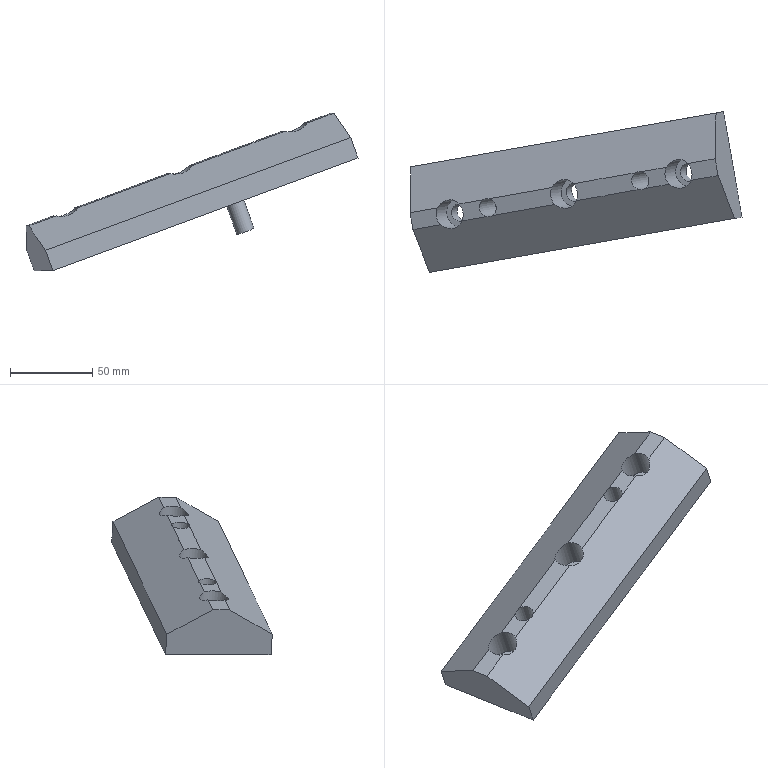Part | NX | features solid 2 | 1 solid | 28 faces | box 201.397 x 97.434 x 95.655 mm | volume 270921 mm3 | plane 17 | cylinder 11 | commonest cylinder face diameters 11 x8 17.5 x3
STEP:
#1=CARTESIAN_POINT('',(972.407,367.24,-198.041));
#2=VERTEX_POINT('',#1);
#3=CARTESIAN_POINT('',(987.359,369.877,-192.515));
#4=VERTEX_POINT('',#3);
#5=CARTESIAN_POINT('',(873.35,349.774,-234.651));
#6=DIRECTION('',(0.9254,0.1632,0.342));
#7=VECTOR('',#6,1000.);
#8=LINE('',#5,#7);
#9=EDGE_CURVE('',#2,#4,#8,.T.);
#10=ORIENTED_EDGE('',*,*,#9,.F.);
#11=CARTESIAN_POINT('',(974.212,357.006,-198.041));
#12=VERTEX_POINT('',#11);
#13=CARTESIAN_POINT('',(966.794,360.974,-200.449));
#14=DIRECTION('',(0.3368,0.05939,-0.9397));
#15=DIRECTION('',(-0.9254,-0.1632,-0.342));
#16=AXIS2_PLACEMENT_3D('',#13,#14,#15);
#17=CIRCLE('',#16,8.75);
#18=EDGE_CURVE('',#2,#12,#17,.T.);
#19=ORIENTED_EDGE('',*,*,#18,.T.);
#20=CARTESIAN_POINT('',(989.164,359.642,-192.515));
#21=VERTEX_POINT('',#20);
#22=CARTESIAN_POINT('',(875.155,339.54,-234.651));
#23=DIRECTION('',(0.9254,0.1632,0.342));
#24=VECTOR('',#23,1000.);
#25=LINE('',#22,#24);
#26=EDGE_CURVE('',#12,#21,#25,.T.);
#27=ORIENTED_EDGE('',*,*,#26,.T.);
#28=CARTESIAN_POINT('',(992.5,360.231,-191.282));
#29=VERTEX_POINT('',#28);
#30=CARTESIAN_POINT('',(989.93,365.054,-191.898));
#31=DIRECTION('',(-0.3368,-0.05939,0.9397));
#32=DIRECTION('',(0.9414,0.,0.3374));
#33=AXIS2_PLACEMENT_3D('',#30,#31,#32);
#34=CIRCLE('',#33,5.5);
#35=EDGE_CURVE('',#21,#29,#34,.T.);
#36=ORIENTED_EDGE('',*,*,#35,.T.);
#37=CARTESIAN_POINT('',(1012.299,363.722,-183.964));
#38=VERTEX_POINT('',#37);
#39=CARTESIAN_POINT('',(875.155,339.54,-234.651));
#40=DIRECTION('',(0.9254,0.1632,0.342));
#41=VECTOR('',#40,1000.);
#42=LINE('',#39,#41);
#43=EDGE_CURVE('',#29,#38,#42,.T.);
#44=ORIENTED_EDGE('',*,*,#43,.T.);
#45=CARTESIAN_POINT('',(1010.495,373.956,-183.964));
#46=VERTEX_POINT('',#45);
#47=CARTESIAN_POINT('',(1013.065,369.133,-183.348));
#48=DIRECTION('',(-0.3368,-0.05939,0.9397));
#49=DIRECTION('',(0.9254,0.1632,0.342));
#50=AXIS2_PLACEMENT_3D('',#47,#48,#49);
#51=CIRCLE('',#50,5.5);
#52=EDGE_CURVE('',#46,#38,#51,.T.);
#53=ORIENTED_EDGE('',*,*,#52,.F.);
#54=CARTESIAN_POINT('',(990.696,370.465,-191.282));
#55=VERTEX_POINT('',#54);
#56=CARTESIAN_POINT('',(873.35,349.774,-234.651));
#57=DIRECTION('',(0.9254,0.1632,0.342));
#58=VECTOR('',#57,1000.);
#59=LINE('',#56,#58);
#60=EDGE_CURVE('',#55,#46,#59,.T.);
#61=ORIENTED_EDGE('',*,*,#60,.F.);
#62=CARTESIAN_POINT('',(989.93,365.054,-191.898));
#63=DIRECTION('',(-0.3368,-0.05939,0.9397));
#64=DIRECTION('',(0.9414,0.,0.3374));
#65=AXIS2_PLACEMENT_3D('',#62,#63,#64);
#66=CIRCLE('',#65,5.5);
#67=EDGE_CURVE('',#55,#4,#66,.T.);
#68=ORIENTED_EDGE('',*,*,#67,.T.);
#69=EDGE_LOOP('',(#10,#19,#27,#36,#44,#53,#61,#68));
#70=FACE_BOUND('',#69,.T.);
#71=CARTESIAN_POINT('',(875.155,339.54,-234.651));
#72=DIRECTION('',(-0.3368,-0.05939,0.9397));
#73=DIRECTION('',(-0.9254,-0.1632,-0.342));
#74=AXIS2_PLACEMENT_3D('',#71,#72,#73);
#75=PLANE('',#74);
#76=ADVANCED_FACE('',(#70),#75,.T.);
#77=CARTESIAN_POINT('',(1051.058,375.832,-200.167));
#78=VERTEX_POINT('',#77);
#79=CARTESIAN_POINT('',(1045.969,374.935,-202.048));
#80=DIRECTION('',(0.3368,0.05939,-0.9397));
#81=DIRECTION('',(0.9254,0.1632,0.342));
#82=AXIS2_PLACEMENT_3D('',#79,#80,#81);
#83=CIRCLE('',#82,5.5);
#84=EDGE_CURVE('',#78,#78,#83,.T.);
#85=ORIENTED_EDGE('',*,*,#84,.F.);
#86=EDGE_LOOP('',(#85));
#87=FACE_BOUND('',#86,.T.);
#88=CARTESIAN_POINT('',(1027.923,371.753,-208.718));
#89=VERTEX_POINT('',#88);
#90=CARTESIAN_POINT('',(1022.833,370.855,-210.599));
#91=DIRECTION('',(-0.3368,-0.05939,0.9397));
#92=DIRECTION('',(0.9254,0.1632,0.342));
#93=AXIS2_PLACEMENT_3D('',#90,#91,#92);
#94=CIRCLE('',#93,5.5);
#95=EDGE_CURVE('',#89,#89,#94,.T.);
#96=ORIENTED_EDGE('',*,*,#95,.T.);
#97=EDGE_LOOP('',(#96));
#98=FACE_BOUND('',#97,.T.);
#99=CARTESIAN_POINT('',(981.652,363.594,-225.819));
#100=VERTEX_POINT('',#99);
#101=CARTESIAN_POINT('',(976.562,362.697,-227.7));
#102=DIRECTION('',(0.3368,0.05939,-0.9397));
#103=DIRECTION('',(0.9254,0.1632,0.342));
#104=AXIS2_PLACEMENT_3D('',#101,#102,#103);
#105=CIRCLE('',#104,5.5);
#106=EDGE_CURVE('',#100,#100,#105,.T.);
#107=ORIENTED_EDGE('',*,*,#106,.F.);
#108=EDGE_LOOP('',(#107));
#109=FACE_BOUND('',#108,.T.);
#110=CARTESIAN_POINT('',(889.664,314.373,-261.902));
#111=VERTEX_POINT('',#110);
#112=CARTESIAN_POINT('',(1074.747,347.008,-193.498));
#113=VERTEX_POINT('',#112);
#114=CARTESIAN_POINT('',(889.664,314.373,-261.902));
#115=DIRECTION('',(0.9254,0.1632,0.342));
#116=VECTOR('',#115,1000.);
#117=LINE('',#114,#116);
#118=EDGE_CURVE('',#111,#113,#117,.T.);
#119=ORIENTED_EDGE('',*,*,#118,.F.);
#120=CARTESIAN_POINT('',(878.377,378.385,-261.902));
#121=VERTEX_POINT('',#120);
#122=CARTESIAN_POINT('',(889.664,314.373,-261.902));
#123=DIRECTION('',(-0.1736,0.9848,0.));
#124=VECTOR('',#123,1000.);
#125=LINE('',#122,#124);
#126=EDGE_CURVE('',#111,#121,#125,.T.);
#127=ORIENTED_EDGE('',*,*,#126,.T.);
#128=CARTESIAN_POINT('',(1063.46,411.021,-193.498));
#129=VERTEX_POINT('',#128);
#130=CARTESIAN_POINT('',(878.377,378.385,-261.902));
#131=DIRECTION('',(0.9254,0.1632,0.342));
#132=VECTOR('',#131,1000.);
#133=LINE('',#130,#132);
#134=EDGE_CURVE('',#121,#129,#133,.T.);
#135=ORIENTED_EDGE('',*,*,#134,.T.);
#136=CARTESIAN_POINT('',(1074.747,347.008,-193.498));
#137=DIRECTION('',(-0.1736,0.9848,0.));
#138=VECTOR('',#137,1000.);
#139=LINE('',#136,#138);
#140=EDGE_CURVE('',#113,#129,#139,.T.);
#141=ORIENTED_EDGE('',*,*,#140,.F.);
#142=EDGE_LOOP('',(#119,#127,#135,#141));
#143=FACE_BOUND('',#142,.T.);
#144=CARTESIAN_POINT('',(935.381,355.435,-242.92));
#145=VERTEX_POINT('',#144);
#146=CARTESIAN_POINT('',(930.291,354.538,-244.801));
#147=DIRECTION('',(-0.3368,-0.05939,0.9397));
#148=DIRECTION('',(0.9254,0.1632,0.342));
#149=AXIS2_PLACEMENT_3D('',#146,#147,#148);
#150=CIRCLE('',#149,5.5);
#151=EDGE_CURVE('',#145,#145,#150,.T.);
#152=ORIENTED_EDGE('',*,*,#151,.T.);
#153=EDGE_LOOP('',(#152));
#154=FACE_BOUND('',#153,.T.);
#155=CARTESIAN_POINT('',(912.246,351.356,-251.47));
#156=VERTEX_POINT('',#155);
#157=CARTESIAN_POINT('',(907.156,350.459,-253.351));
#158=DIRECTION('',(0.3368,0.05939,-0.9397));
#159=DIRECTION('',(0.9254,0.1632,0.342));
#160=AXIS2_PLACEMENT_3D('',#157,#158,#159);
#161=CIRCLE('',#160,5.5);
#162=EDGE_CURVE('',#156,#156,#161,.T.);
#163=ORIENTED_EDGE('',*,*,#162,.F.);
#164=EDGE_LOOP('',(#163));
#165=FACE_BOUND('',#164,.T.);
#166=CARTESIAN_POINT('',(1004.875,366.776,-217.294));
#167=VERTEX_POINT('',#166);
#168=CARTESIAN_POINT('',(999.698,366.776,-219.149));
#169=DIRECTION('',(-0.3368,-0.05939,0.9397));
#170=DIRECTION('',(0.9414,0.,0.3374));
#171=AXIS2_PLACEMENT_3D('',#168,#169,#170);
#172=CIRCLE('',#171,5.5);
#173=EDGE_CURVE('',#167,#167,#172,.T.);
#174=ORIENTED_EDGE('',*,*,#173,.T.);
#175=EDGE_LOOP('',(#174));
#176=FACE_BOUND('',#175,.T.);
#177=CARTESIAN_POINT('',(889.664,314.373,-261.902));
#178=DIRECTION('',(-0.3368,-0.05939,0.9397));
#179=DIRECTION('',(0.1736,-0.9848,0.));
#180=AXIS2_PLACEMENT_3D('',#177,#178,#179);
#181=PLANE('',#180);
#182=ADVANCED_FACE('',(#87,#98,#109,#143,#154,#165,#176),#181,.F.);
#183=ORIENTED_EDGE('',*,*,#60,.T.);
#184=CARTESIAN_POINT('',(1013.831,374.545,-182.731));
#185=VERTEX_POINT('',#184);
#186=CARTESIAN_POINT('',(1012.055,368.955,-180.529));
#187=DIRECTION('',(0.3785,-0.441,-0.8138));
#188=DIRECTION('',(0.01803,0.8826,-0.4698));
#189=AXIS2_PLACEMENT_3D('',#186,#187,#188);
#190=ELLIPSE('',#189,6.351,5.5);
#191=EDGE_CURVE('',#46,#185,#190,.T.);
#192=ORIENTED_EDGE('',*,*,#191,.T.);
#193=CARTESIAN_POINT('',(1028.783,377.181,-177.205));
#194=VERTEX_POINT('',#193);
#195=CARTESIAN_POINT('',(873.35,349.774,-234.651));
#196=DIRECTION('',(0.9254,0.1632,0.342));
#197=VECTOR('',#196,1000.);
#198=LINE('',#195,#197);
#199=EDGE_CURVE('',#185,#194,#198,.T.);
#200=ORIENTED_EDGE('',*,*,#199,.T.);
#201=CARTESIAN_POINT('',(1041.813,379.479,-172.389));
#202=VERTEX_POINT('',#201);
#203=CARTESIAN_POINT('',(1035.19,373.034,-171.978));
#204=DIRECTION('',(0.3785,-0.441,-0.8138));
#205=DIRECTION('',(0.01803,0.8826,-0.4698));
#206=AXIS2_PLACEMENT_3D('',#203,#204,#205);
#207=ELLIPSE('',#206,10.104,8.75);
#208=EDGE_CURVE('',#194,#202,#207,.T.);
#209=ORIENTED_EDGE('',*,*,#208,.T.);
#210=CARTESIAN_POINT('',(1058.434,382.409,-166.247));
#211=VERTEX_POINT('',#210);
#212=CARTESIAN_POINT('',(873.35,349.774,-234.651));
#213=DIRECTION('',(0.9254,0.1632,0.342));
#214=VECTOR('',#213,1000.);
#215=LINE('',#212,#214);
#216=EDGE_CURVE('',#202,#211,#215,.T.);
#217=ORIENTED_EDGE('',*,*,#216,.T.);
#218=CARTESIAN_POINT('',(1059.002,410.234,-181.06));
#219=VERTEX_POINT('',#218);
#220=CARTESIAN_POINT('',(1058.434,382.409,-166.247));
#221=DIRECTION('',(0.01803,0.8826,-0.4698));
#222=VECTOR('',#221,1000.);
#223=LINE('',#220,#222);
#224=EDGE_CURVE('',#211,#219,#223,.T.);
#225=ORIENTED_EDGE('',*,*,#224,.T.);
#226=CARTESIAN_POINT('',(873.919,377.599,-249.464));
#227=VERTEX_POINT('',#226);
#228=CARTESIAN_POINT('',(873.919,377.599,-249.464));
#229=DIRECTION('',(0.9254,0.1632,0.342));
#230=VECTOR('',#229,1000.);
#231=LINE('',#228,#230);
#232=EDGE_CURVE('',#227,#219,#231,.T.);
#233=ORIENTED_EDGE('',*,*,#232,.F.);
#234=CARTESIAN_POINT('',(873.35,349.774,-234.651));
#235=VERTEX_POINT('',#234);
#236=CARTESIAN_POINT('',(873.35,349.774,-234.651));
#237=DIRECTION('',(0.01803,0.8826,-0.4698));
#238=VECTOR('',#237,1000.);
#239=LINE('',#236,#238);
#240=EDGE_CURVE('',#235,#227,#239,.T.);
#241=ORIENTED_EDGE('',*,*,#240,.F.);
#242=CARTESIAN_POINT('',(889.971,352.705,-228.508));
#243=VERTEX_POINT('',#242);
#244=CARTESIAN_POINT('',(873.35,349.774,-234.651));
#245=DIRECTION('',(0.9254,0.1632,0.342));
#246=VECTOR('',#245,1000.);
#247=LINE('',#244,#246);
#248=EDGE_CURVE('',#235,#243,#247,.T.);
#249=ORIENTED_EDGE('',*,*,#248,.T.);
#250=CARTESIAN_POINT('',(903.001,355.002,-223.692));
#251=VERTEX_POINT('',#250);
#252=CARTESIAN_POINT('',(896.378,348.558,-223.281));
#253=DIRECTION('',(0.3785,-0.441,-0.8138));
#254=DIRECTION('',(0.01803,0.8826,-0.4698));
#255=AXIS2_PLACEMENT_3D('',#252,#253,#254);
#256=ELLIPSE('',#255,10.104,8.75);
#257=EDGE_CURVE('',#243,#251,#256,.T.);
#258=ORIENTED_EDGE('',*,*,#257,.T.);
#259=CARTESIAN_POINT('',(917.953,357.639,-218.166));
#260=VERTEX_POINT('',#259);
#261=CARTESIAN_POINT('',(873.35,349.774,-234.651));
#262=DIRECTION('',(0.9254,0.1632,0.342));
#263=VECTOR('',#262,1000.);
#264=LINE('',#261,#263);
#265=EDGE_CURVE('',#251,#260,#264,.T.);
#266=ORIENTED_EDGE('',*,*,#265,.T.);
#267=CARTESIAN_POINT('',(921.29,358.227,-216.933));
#268=VERTEX_POINT('',#267);
#269=CARTESIAN_POINT('',(919.513,352.637,-214.731));
#270=DIRECTION('',(0.3785,-0.441,-0.8138));
#271=DIRECTION('',(0.01803,0.8826,-0.4698));
#272=AXIS2_PLACEMENT_3D('',#269,#270,#271);
#273=ELLIPSE('',#272,6.351,5.5);
#274=EDGE_CURVE('',#260,#268,#273,.T.);
#275=ORIENTED_EDGE('',*,*,#274,.T.);
#276=CARTESIAN_POINT('',(959.377,364.943,-202.857));
#277=VERTEX_POINT('',#276);
#278=CARTESIAN_POINT('',(873.35,349.774,-234.651));
#279=DIRECTION('',(0.9254,0.1632,0.342));
#280=VECTOR('',#279,1000.);
#281=LINE('',#278,#280);
#282=EDGE_CURVE('',#268,#277,#281,.T.);
#283=ORIENTED_EDGE('',*,*,#282,.T.);
#284=CARTESIAN_POINT('',(965.784,360.796,-197.63));
#285=DIRECTION('',(0.3785,-0.441,-0.8138));
#286=DIRECTION('',(0.01803,0.8826,-0.4698));
#287=AXIS2_PLACEMENT_3D('',#284,#285,#286);
#288=ELLIPSE('',#287,10.104,8.75);
#289=EDGE_CURVE('',#277,#2,#288,.T.);
#290=ORIENTED_EDGE('',*,*,#289,.T.);
#291=ORIENTED_EDGE('',*,*,#9,.T.);
#292=CARTESIAN_POINT('',(988.919,364.876,-189.079));
#293=DIRECTION('',(-0.3785,0.441,0.8138));
#294=DIRECTION('',(0.01803,0.8826,-0.4698));
#295=AXIS2_PLACEMENT_3D('',#292,#293,#294);
#296=ELLIPSE('',#295,6.351,5.5);
#297=EDGE_CURVE('',#4,#55,#296,.F.);
#298=ORIENTED_EDGE('',*,*,#297,.T.);
#299=EDGE_LOOP('',(#183,#192,#200,#209,#217,#225,#233,#241,#249,#258,#266,#275,#283,#290,#291,#298));
#300=FACE_BOUND('',#299,.T.);
#301=CARTESIAN_POINT('',(873.35,349.774,-234.651));
#302=DIRECTION('',(-0.3785,0.441,0.8138));
#303=DIRECTION('',(-0.01803,-0.8826,0.4698));
#304=AXIS2_PLACEMENT_3D('',#301,#302,#303);
#305=PLANE('',#304);
#306=ADVANCED_FACE('',(#300),#305,.T.);
#307=ORIENTED_EDGE('',*,*,#26,.F.);
#308=CARTESIAN_POINT('',(961.182,354.708,-202.857));
#309=VERTEX_POINT('',#308);
#310=CARTESIAN_POINT('',(965.784,360.796,-197.63));
#311=DIRECTION('',(-0.2049,-0.5438,0.8138));
#312=DIRECTION('',(0.3188,-0.8232,-0.4698));
#313=AXIS2_PLACEMENT_3D('',#310,#311,#312);
#314=ELLIPSE('',#313,10.104,8.75);
#315=EDGE_CURVE('',#309,#12,#314,.T.);
#316=ORIENTED_EDGE('',*,*,#315,.F.);
#317=CARTESIAN_POINT('',(923.094,347.993,-216.933));
#318=VERTEX_POINT('',#317);
#319=CARTESIAN_POINT('',(875.155,339.54,-234.651));
#320=DIRECTION('',(0.9254,0.1632,0.342));
#321=VECTOR('',#320,1000.);
#322=LINE('',#319,#321);
#323=EDGE_CURVE('',#318,#309,#322,.T.);
#324=ORIENTED_EDGE('',*,*,#323,.F.);
#325=CARTESIAN_POINT('',(919.758,347.404,-218.166));
#326=VERTEX_POINT('',#325);
#327=CARTESIAN_POINT('',(919.513,352.637,-214.731));
#328=DIRECTION('',(-0.2049,-0.5438,0.8138));
#329=DIRECTION('',(0.3188,-0.8232,-0.4698));
#330=AXIS2_PLACEMENT_3D('',#327,#328,#329);
#331=ELLIPSE('',#330,6.351,5.5);
#332=EDGE_CURVE('',#326,#318,#331,.T.);
#333=ORIENTED_EDGE('',*,*,#332,.F.);
#334=CARTESIAN_POINT('',(904.805,344.768,-223.692));
#335=VERTEX_POINT('',#334);
#336=CARTESIAN_POINT('',(875.155,339.54,-234.651));
#337=DIRECTION('',(0.9254,0.1632,0.342));
#338=VECTOR('',#337,1000.);
#339=LINE('',#336,#338);
#340=EDGE_CURVE('',#335,#326,#339,.T.);
#341=ORIENTED_EDGE('',*,*,#340,.F.);
#342=CARTESIAN_POINT('',(891.775,342.47,-228.508));
#343=VERTEX_POINT('',#342);
#344=CARTESIAN_POINT('',(896.378,348.558,-223.281));
#345=DIRECTION('',(-0.2049,-0.5438,0.8138));
#346=DIRECTION('',(0.3188,-0.8232,-0.4698));
#347=AXIS2_PLACEMENT_3D('',#344,#345,#346);
#348=ELLIPSE('',#347,10.104,8.75);
#349=EDGE_CURVE('',#343,#335,#348,.T.);
#350=ORIENTED_EDGE('',*,*,#349,.F.);
#351=CARTESIAN_POINT('',(875.155,339.54,-234.651));
#352=VERTEX_POINT('',#351);
#353=CARTESIAN_POINT('',(875.155,339.54,-234.651));
#354=DIRECTION('',(0.9254,0.1632,0.342));
#355=VECTOR('',#354,1000.);
#356=LINE('',#353,#355);
#357=EDGE_CURVE('',#352,#343,#356,.T.);
#358=ORIENTED_EDGE('',*,*,#357,.F.);
#359=CARTESIAN_POINT('',(885.206,313.587,-249.464));
#360=VERTEX_POINT('',#359);
#361=CARTESIAN_POINT('',(875.155,339.54,-234.651));
#362=DIRECTION('',(0.3188,-0.8232,-0.4698));
#363=VECTOR('',#362,1000.);
#364=LINE('',#361,#363);
#365=EDGE_CURVE('',#352,#360,#364,.T.);
#366=ORIENTED_EDGE('',*,*,#365,.T.);
#367=CARTESIAN_POINT('',(1070.289,346.222,-181.06));
#368=VERTEX_POINT('',#367);
#369=CARTESIAN_POINT('',(885.206,313.587,-249.464));
#370=DIRECTION('',(0.9254,0.1632,0.342));
#371=VECTOR('',#370,1000.);
#372=LINE('',#369,#371);
#373=EDGE_CURVE('',#360,#368,#372,.T.);
#374=ORIENTED_EDGE('',*,*,#373,.T.);
#375=CARTESIAN_POINT('',(1060.238,372.175,-166.247));
#376=VERTEX_POINT('',#375);
#377=CARTESIAN_POINT('',(1060.238,372.175,-166.247));
#378=DIRECTION('',(0.3188,-0.8232,-0.4698));
#379=VECTOR('',#378,1000.);
#380=LINE('',#377,#379);
#381=EDGE_CURVE('',#376,#368,#380,.T.);
#382=ORIENTED_EDGE('',*,*,#381,.F.);
#383=CARTESIAN_POINT('',(1043.618,369.244,-172.389));
#384=VERTEX_POINT('',#383);
#385=CARTESIAN_POINT('',(875.155,339.54,-234.651));
#386=DIRECTION('',(0.9254,0.1632,0.342));
#387=VECTOR('',#386,1000.);
#388=LINE('',#385,#387);
#389=EDGE_CURVE('',#384,#376,#388,.T.);
#390=ORIENTED_EDGE('',*,*,#389,.F.);
#391=CARTESIAN_POINT('',(1030.588,366.947,-177.205));
#392=VERTEX_POINT('',#391);
#393=CARTESIAN_POINT('',(1035.19,373.034,-171.978));
#394=DIRECTION('',(-0.2049,-0.5438,0.8138));
#395=DIRECTION('',(0.3188,-0.8232,-0.4698));
#396=AXIS2_PLACEMENT_3D('',#393,#394,#395);
#397=ELLIPSE('',#396,10.104,8.75);
#398=EDGE_CURVE('',#392,#384,#397,.T.);
#399=ORIENTED_EDGE('',*,*,#398,.F.);
#400=CARTESIAN_POINT('',(1015.636,364.31,-182.731));
#401=VERTEX_POINT('',#400);
#402=CARTESIAN_POINT('',(875.155,339.54,-234.651));
#403=DIRECTION('',(0.9254,0.1632,0.342));
#404=VECTOR('',#403,1000.);
#405=LINE('',#402,#404);
#406=EDGE_CURVE('',#401,#392,#405,.T.);
#407=ORIENTED_EDGE('',*,*,#406,.F.);
#408=CARTESIAN_POINT('',(1012.055,368.955,-180.529));
#409=DIRECTION('',(-0.2049,-0.5438,0.8138));
#410=DIRECTION('',(0.3188,-0.8232,-0.4698));
#411=AXIS2_PLACEMENT_3D('',#408,#409,#410);
#412=ELLIPSE('',#411,6.351,5.5);
#413=EDGE_CURVE('',#38,#401,#412,.T.);
#414=ORIENTED_EDGE('',*,*,#413,.F.);
#415=ORIENTED_EDGE('',*,*,#43,.F.);
#416=CARTESIAN_POINT('',(988.919,364.876,-189.079));
#417=DIRECTION('',(-0.2049,-0.5438,0.8138));
#418=DIRECTION('',(0.3188,-0.8232,-0.4698));
#419=AXIS2_PLACEMENT_3D('',#416,#417,#418);
#420=ELLIPSE('',#419,6.351,5.5);
#421=EDGE_CURVE('',#29,#21,#420,.F.);
#422=ORIENTED_EDGE('',*,*,#421,.T.);
#423=EDGE_LOOP('',(#307,#316,#324,#333,#341,#350,#358,#366,#374,#382,#390,#399,#407,#414,#415,#422));
#424=FACE_BOUND('',#423,.T.);
#425=CARTESIAN_POINT('',(875.155,339.54,-234.651));
#426=DIRECTION('',(-0.2049,-0.5438,0.8138));
#427=DIRECTION('',(-0.3188,0.8232,0.4698));
#428=AXIS2_PLACEMENT_3D('',#425,#426,#427);
#429=PLANE('',#428);
#430=ADVANCED_FACE('',(#424),#429,.T.);
#431=CARTESIAN_POINT('',(966.794,360.974,-200.449));
#432=DIRECTION('',(-0.3368,-0.05939,0.9397));
#433=DIRECTION('',(0.9254,0.1632,0.342));
#434=AXIS2_PLACEMENT_3D('',#431,#432,#433);
#435=CIRCLE('',#434,8.75);
#436=EDGE_CURVE('',#277,#309,#435,.T.);
#437=ORIENTED_EDGE('',*,*,#436,.F.);
#438=ORIENTED_EDGE('',*,*,#282,.F.);
#439=CARTESIAN_POINT('',(920.524,352.816,-217.55));
#440=DIRECTION('',(-0.3368,-0.05939,0.9397));
#441=DIRECTION('',(0.9254,0.1632,0.342));
#442=AXIS2_PLACEMENT_3D('',#439,#440,#441);
#443=CIRCLE('',#442,5.5);
#444=EDGE_CURVE('',#318,#268,#443,.T.);
#445=ORIENTED_EDGE('',*,*,#444,.F.);
#446=ORIENTED_EDGE('',*,*,#323,.T.);
#447=EDGE_LOOP('',(#437,#438,#445,#446));
#448=FACE_BOUND('',#447,.T.);
#449=CARTESIAN_POINT('',(875.155,339.54,-234.651));
#450=DIRECTION('',(-0.3368,-0.05939,0.9397));
#451=DIRECTION('',(-0.9254,-0.1632,-0.342));
#452=AXIS2_PLACEMENT_3D('',#449,#450,#451);
#453=PLANE('',#452);
#454=ADVANCED_FACE('',(#448),#453,.T.);
#455=CARTESIAN_POINT('',(920.524,352.816,-217.55));
#456=DIRECTION('',(-0.3368,-0.05939,0.9397));
#457=DIRECTION('',(0.9254,0.1632,0.342));
#458=AXIS2_PLACEMENT_3D('',#455,#456,#457);
#459=CIRCLE('',#458,5.5);
#460=EDGE_CURVE('',#260,#326,#459,.T.);
#461=ORIENTED_EDGE('',*,*,#460,.F.);
#462=ORIENTED_EDGE('',*,*,#265,.F.);
#463=CARTESIAN_POINT('',(897.388,348.736,-226.1));
#464=DIRECTION('',(0.3368,0.05939,-0.9397));
#465=DIRECTION('',(-0.9254,-0.1632,-0.342));
#466=AXIS2_PLACEMENT_3D('',#463,#464,#465);
#467=CIRCLE('',#466,8.75);
#468=EDGE_CURVE('',#251,#335,#467,.T.);
#469=ORIENTED_EDGE('',*,*,#468,.T.);
#470=ORIENTED_EDGE('',*,*,#340,.T.);
#471=EDGE_LOOP('',(#461,#462,#469,#470));
#472=FACE_BOUND('',#471,.T.);
#473=CARTESIAN_POINT('',(875.155,339.54,-234.651));
#474=DIRECTION('',(-0.3368,-0.05939,0.9397));
#475=DIRECTION('',(-0.9254,-0.1632,-0.342));
#476=AXIS2_PLACEMENT_3D('',#473,#474,#475);
#477=PLANE('',#476);
#478=ADVANCED_FACE('',(#472),#477,.T.);
#479=CARTESIAN_POINT('',(1036.201,373.213,-174.797));
#480=DIRECTION('',(-0.3368,-0.05939,0.9397));
#481=DIRECTION('',(0.9254,0.1632,0.342));
#482=AXIS2_PLACEMENT_3D('',#479,#480,#481);
#483=CIRCLE('',#482,8.75);
#484=EDGE_CURVE('',#194,#392,#483,.T.);
#485=ORIENTED_EDGE('',*,*,#484,.F.);
#486=ORIENTED_EDGE('',*,*,#199,.F.);
#487=CARTESIAN_POINT('',(1013.065,369.133,-183.348));
#488=DIRECTION('',(0.3368,0.05939,-0.9397));
#489=DIRECTION('',(-0.9254,-0.1632,-0.342));
#490=AXIS2_PLACEMENT_3D('',#487,#488,#489);
#491=CIRCLE('',#490,5.5);
#492=EDGE_CURVE('',#185,#401,#491,.T.);
#493=ORIENTED_EDGE('',*,*,#492,.T.);
#494=ORIENTED_EDGE('',*,*,#406,.T.);
#495=EDGE_LOOP('',(#485,#486,#493,#494));
#496=FACE_BOUND('',#495,.T.);
#497=CARTESIAN_POINT('',(875.155,339.54,-234.651));
#498=DIRECTION('',(-0.3368,-0.05939,0.9397));
#499=DIRECTION('',(-0.9254,-0.1632,-0.342));
#500=AXIS2_PLACEMENT_3D('',#497,#498,#499);
#501=PLANE('',#500);
#502=ADVANCED_FACE('',(#496),#501,.T.);
#503=CARTESIAN_POINT('',(1060.238,372.175,-166.247));
#504=DIRECTION('',(-0.1736,0.9848,0.));
#505=VECTOR('',#504,1000.);
#506=LINE('',#503,#505);
#507=EDGE_CURVE('',#376,#211,#506,.T.);
#508=ORIENTED_EDGE('',*,*,#507,.T.);
#509=ORIENTED_EDGE('',*,*,#216,.F.);
#510=CARTESIAN_POINT('',(1036.201,373.213,-174.797));
#511=DIRECTION('',(0.3368,0.05939,-0.9397));
#512=DIRECTION('',(-0.9254,-0.1632,-0.342));
#513=AXIS2_PLACEMENT_3D('',#510,#511,#512);
#514=CIRCLE('',#513,8.75);
#515=EDGE_CURVE('',#202,#384,#514,.T.);
#516=ORIENTED_EDGE('',*,*,#515,.T.);
#517=ORIENTED_EDGE('',*,*,#389,.T.);
#518=EDGE_LOOP('',(#508,#509,#516,#517));
#519=FACE_BOUND('',#518,.T.);
#520=CARTESIAN_POINT('',(875.155,339.54,-234.651));
#521=DIRECTION('',(-0.3368,-0.05939,0.9397));
#522=DIRECTION('',(-0.9254,-0.1632,-0.342));
#523=AXIS2_PLACEMENT_3D('',#520,#521,#522);
#524=PLANE('',#523);
#525=ADVANCED_FACE('',(#519),#524,.T.);
#526=CARTESIAN_POINT('',(897.388,348.736,-226.1));
#527=DIRECTION('',(-0.3368,-0.05939,0.9397));
#528=DIRECTION('',(0.9254,0.1632,0.342));
#529=AXIS2_PLACEMENT_3D('',#526,#527,#528);
#530=CIRCLE('',#529,8.75);
#531=EDGE_CURVE('',#243,#343,#530,.T.);
#532=ORIENTED_EDGE('',*,*,#531,.F.);
#533=ORIENTED_EDGE('',*,*,#248,.F.);
#534=CARTESIAN_POINT('',(875.155,339.54,-234.651));
#535=DIRECTION('',(-0.1736,0.9848,0.));
#536=VECTOR('',#535,1000.);
#537=LINE('',#534,#536);
#538=EDGE_CURVE('',#352,#235,#537,.T.);
#539=ORIENTED_EDGE('',*,*,#538,.F.);
#540=ORIENTED_EDGE('',*,*,#357,.T.);
#541=EDGE_LOOP('',(#532,#533,#539,#540));
#542=FACE_BOUND('',#541,.T.);
#543=CARTESIAN_POINT('',(875.155,339.54,-234.651));
#544=DIRECTION('',(-0.3368,-0.05939,0.9397));
#545=DIRECTION('',(-0.9254,-0.1632,-0.342));
#546=AXIS2_PLACEMENT_3D('',#543,#544,#545);
#547=PLANE('',#546);
#548=ADVANCED_FACE('',(#542),#547,.T.);
#549=ORIENTED_EDGE('',*,*,#538,.T.);
#550=ORIENTED_EDGE('',*,*,#240,.T.);
#551=CARTESIAN_POINT('',(883.429,379.276,-275.997));
#552=DIRECTION('',(-0.3368,-0.05939,0.9397));
#553=VECTOR('',#552,1000.);
#554=LINE('',#551,#553);
#555=EDGE_CURVE('',#121,#227,#554,.T.);
#556=ORIENTED_EDGE('',*,*,#555,.F.);
#557=ORIENTED_EDGE('',*,*,#126,.F.);
#558=CARTESIAN_POINT('',(894.717,315.264,-275.997));
#559=DIRECTION('',(-0.3368,-0.05939,0.9397));
#560=VECTOR('',#559,1000.);
#561=LINE('',#558,#560);
#562=EDGE_CURVE('',#111,#360,#561,.T.);
#563=ORIENTED_EDGE('',*,*,#562,.T.);
#564=ORIENTED_EDGE('',*,*,#365,.F.);
#565=EDGE_LOOP('',(#549,#550,#556,#557,#563,#564));
#566=FACE_BOUND('',#565,.T.);
#567=CARTESIAN_POINT('',(873.242,344.479,-231.832));
#568=DIRECTION('',(-0.9254,-0.1632,-0.342));
#569=DIRECTION('',(0.3368,0.05939,-0.9397));
#570=AXIS2_PLACEMENT_3D('',#567,#568,#569);
#571=PLANE('',#570);
#572=ADVANCED_FACE('',(#566),#571,.T.);
#573=ORIENTED_EDGE('',*,*,#507,.F.);
#574=ORIENTED_EDGE('',*,*,#381,.T.);
#575=CARTESIAN_POINT('',(1079.8,347.899,-207.593));
#576=DIRECTION('',(-0.3368,-0.05939,0.9397));
#577=VECTOR('',#576,1000.);
#578=LINE('',#575,#577);
#579=EDGE_CURVE('',#113,#368,#578,.T.);
#580=ORIENTED_EDGE('',*,*,#579,.F.);
#581=ORIENTED_EDGE('',*,*,#140,.T.);
#582=CARTESIAN_POINT('',(1068.513,411.911,-207.593));
#583=DIRECTION('',(-0.3368,-0.05939,0.9397));
#584=VECTOR('',#583,1000.);
#585=LINE('',#582,#584);
#586=EDGE_CURVE('',#129,#219,#585,.T.);
#587=ORIENTED_EDGE('',*,*,#586,.T.);
#588=ORIENTED_EDGE('',*,*,#224,.F.);
#589=EDGE_LOOP('',(#573,#574,#580,#581,#587,#588));
#590=FACE_BOUND('',#589,.T.);
#591=CARTESIAN_POINT('',(1058.326,377.114,-163.428));
#592=DIRECTION('',(-0.9254,-0.1632,-0.342));
#593=DIRECTION('',(0.3368,0.05939,-0.9397));
#594=AXIS2_PLACEMENT_3D('',#591,#592,#593);
#595=PLANE('',#594);
#596=ADVANCED_FACE('',(#590),#595,.F.);
#597=ORIENTED_EDGE('',*,*,#84,.T.);
#598=EDGE_LOOP('',(#597));
#599=FACE_BOUND('',#598,.T.);
#600=CARTESIAN_POINT('',(1037.423,374.341,-194.507));
#601=VERTEX_POINT('',#600);
#602=CARTESIAN_POINT('',(1042.6,374.341,-192.651));
#603=DIRECTION('',(0.3368,0.05939,-0.9397));
#604=DIRECTION('',(-0.9414,0.,-0.3374));
#605=AXIS2_PLACEMENT_3D('',#602,#603,#604);
#606=CIRCLE('',#605,5.5);
#607=EDGE_CURVE('',#601,#601,#606,.F.);
#608=ORIENTED_EDGE('',*,*,#607,.T.);
#609=EDGE_LOOP('',(#608));
#610=FACE_BOUND('',#609,.T.);
#611=CARTESIAN_POINT('',(1052.031,376.004,-218.963));
#612=DIRECTION('',(0.3368,0.05939,-0.9397));
#613=DIRECTION('',(0.9254,0.1632,0.342));
#614=AXIS2_PLACEMENT_3D('',#611,#612,#613);
#615=CYLINDRICAL_SURFACE('',#614,5.5);
#616=ADVANCED_FACE('',(#599,#610),#615,.F.);
#617=ORIENTED_EDGE('',*,*,#607,.F.);
#618=EDGE_LOOP('',(#617));
#619=FACE_BOUND('',#618,.T.);
#620=CARTESIAN_POINT('',(1034.363,374.341,-195.604));
#621=VERTEX_POINT('',#620);
#622=CARTESIAN_POINT('',(1042.6,374.341,-192.651));
#623=DIRECTION('',(0.3368,0.05939,-0.9397));
#624=DIRECTION('',(-0.9414,0.,-0.3374));
#625=AXIS2_PLACEMENT_3D('',#622,#623,#624);
#626=CIRCLE('',#625,8.75);
#627=EDGE_CURVE('',#621,#621,#626,.F.);
#628=ORIENTED_EDGE('',*,*,#627,.T.);
#629=EDGE_LOOP('',(#628));
#630=FACE_BOUND('',#629,.T.);
#631=CARTESIAN_POINT('',(996.329,366.182,-209.752));
#632=DIRECTION('',(0.3368,0.05939,-0.9397));
#633=DIRECTION('',(0.9254,0.1632,0.342));
#634=AXIS2_PLACEMENT_3D('',#631,#632,#633);
#635=PLANE('',#634);
#636=ADVANCED_FACE('',(#619,#630),#635,.F.);
#637=ORIENTED_EDGE('',*,*,#627,.F.);
#638=EDGE_LOOP('',(#637));
#639=FACE_BOUND('',#638,.T.);
#640=ORIENTED_EDGE('',*,*,#484,.T.);
#641=ORIENTED_EDGE('',*,*,#398,.T.);
#642=ORIENTED_EDGE('',*,*,#515,.F.);
#643=ORIENTED_EDGE('',*,*,#208,.F.);
#644=EDGE_LOOP('',(#640,#641,#642,#643));
#645=FACE_BOUND('',#644,.T.);
#646=CARTESIAN_POINT('',(1036.201,373.213,-174.797));
#647=DIRECTION('',(0.3368,0.05939,-0.9397));
#648=DIRECTION('',(0.9254,0.1632,0.342));
#649=AXIS2_PLACEMENT_3D('',#646,#647,#648);
#650=CYLINDRICAL_SURFACE('',#649,8.75);
#651=ADVANCED_FACE('',(#639,#645),#650,.F.);
#652=ORIENTED_EDGE('',*,*,#95,.F.);
#653=EDGE_LOOP('',(#652));
#654=FACE_BOUND('',#653,.T.);
#655=ORIENTED_EDGE('',*,*,#52,.T.);
#656=ORIENTED_EDGE('',*,*,#413,.T.);
#657=ORIENTED_EDGE('',*,*,#492,.F.);
#658=ORIENTED_EDGE('',*,*,#191,.F.);
#659=EDGE_LOOP('',(#655,#656,#657,#658));
#660=FACE_BOUND('',#659,.T.);
#661=CARTESIAN_POINT('',(1013.065,369.133,-183.348));
#662=DIRECTION('',(0.3368,0.05939,-0.9397));
#663=DIRECTION('',(0.9254,0.1632,0.342));
#664=AXIS2_PLACEMENT_3D('',#661,#662,#663);
#665=CYLINDRICAL_SURFACE('',#664,5.5);
#666=ADVANCED_FACE('',(#654,#660),#665,.F.);
#667=ORIENTED_EDGE('',*,*,#106,.T.);
#668=EDGE_LOOP('',(#667));
#669=FACE_BOUND('',#668,.T.);
#670=CARTESIAN_POINT('',(968.017,362.103,-220.159));
#671=VERTEX_POINT('',#670);
#672=CARTESIAN_POINT('',(973.194,362.103,-218.303));
#673=DIRECTION('',(0.3368,0.05939,-0.9397));
#674=DIRECTION('',(-0.9414,0.,-0.3374));
#675=AXIS2_PLACEMENT_3D('',#672,#673,#674);
#676=CIRCLE('',#675,5.5);
#677=EDGE_CURVE('',#671,#671,#676,.F.);
#678=ORIENTED_EDGE('',*,*,#677,.T.);
#679=EDGE_LOOP('',(#678));
#680=FACE_BOUND('',#679,.T.);
#681=CARTESIAN_POINT('',(982.625,363.766,-244.614));
#682=DIRECTION('',(0.3368,0.05939,-0.9397));
#683=DIRECTION('',(0.9254,0.1632,0.342));
#684=AXIS2_PLACEMENT_3D('',#681,#682,#683);
#685=CYLINDRICAL_SURFACE('',#684,5.5);
#686=ADVANCED_FACE('',(#669,#680),#685,.F.);
#687=ORIENTED_EDGE('',*,*,#677,.F.);
#688=EDGE_LOOP('',(#687));
#689=FACE_BOUND('',#688,.T.);
#690=CARTESIAN_POINT('',(964.957,362.103,-221.255));
#691=VERTEX_POINT('',#690);
#692=CARTESIAN_POINT('',(973.194,362.103,-218.303));
#693=DIRECTION('',(0.3368,0.05939,-0.9397));
#694=DIRECTION('',(-0.9414,0.,-0.3374));
#695=AXIS2_PLACEMENT_3D('',#692,#693,#694);
#696=CIRCLE('',#695,8.75);
#697=EDGE_CURVE('',#691,#691,#696,.F.);
#698=ORIENTED_EDGE('',*,*,#697,.T.);
#699=EDGE_LOOP('',(#698));
#700=FACE_BOUND('',#699,.T.);
#701=CARTESIAN_POINT('',(973.194,362.103,-218.303));
#702=DIRECTION('',(0.3368,0.05939,-0.9397));
#703=DIRECTION('',(0.9254,0.1632,0.342));
#704=AXIS2_PLACEMENT_3D('',#701,#702,#703);
#705=PLANE('',#704);
#706=ADVANCED_FACE('',(#689,#700),#705,.F.);
#707=ORIENTED_EDGE('',*,*,#697,.F.);
#708=EDGE_LOOP('',(#707));
#709=FACE_BOUND('',#708,.T.);
#710=ORIENTED_EDGE('',*,*,#436,.T.);
#711=ORIENTED_EDGE('',*,*,#315,.T.);
#712=ORIENTED_EDGE('',*,*,#18,.F.);
#713=ORIENTED_EDGE('',*,*,#289,.F.);
#714=EDGE_LOOP('',(#710,#711,#712,#713));
#715=FACE_BOUND('',#714,.T.);
#716=CARTESIAN_POINT('',(966.794,360.974,-200.449));
#717=DIRECTION('',(0.3368,0.05939,-0.9397));
#718=DIRECTION('',(0.9254,0.1632,0.342));
#719=AXIS2_PLACEMENT_3D('',#716,#717,#718);
#720=CYLINDRICAL_SURFACE('',#719,8.75);
#721=ADVANCED_FACE('',(#709,#715),#720,.F.);
#722=CARTESIAN_POINT('',(898.61,349.865,-245.81));
#723=VERTEX_POINT('',#722);
#724=CARTESIAN_POINT('',(903.788,349.865,-243.954));
#725=DIRECTION('',(0.3368,0.05939,-0.9397));
#726=DIRECTION('',(-0.9414,0.,-0.3374));
#727=AXIS2_PLACEMENT_3D('',#724,#725,#726);
#728=CIRCLE('',#727,5.5);
#729=EDGE_CURVE('',#723,#723,#728,.F.);
#730=ORIENTED_EDGE('',*,*,#729,.T.);
#731=EDGE_LOOP('',(#730));
#732=FACE_BOUND('',#731,.T.);
#733=ORIENTED_EDGE('',*,*,#162,.T.);
#734=EDGE_LOOP('',(#733));
#735=FACE_BOUND('',#734,.T.);
#736=CARTESIAN_POINT('',(913.219,351.528,-270.266));
#737=DIRECTION('',(0.3368,0.05939,-0.9397));
#738=DIRECTION('',(0.9254,0.1632,0.342));
#739=AXIS2_PLACEMENT_3D('',#736,#737,#738);
#740=CYLINDRICAL_SURFACE('',#739,5.5);
#741=ADVANCED_FACE('',(#732,#735),#740,.F.);
#742=CARTESIAN_POINT('',(895.551,349.865,-246.907));
#743=VERTEX_POINT('',#742);
#744=CARTESIAN_POINT('',(903.788,349.865,-243.954));
#745=DIRECTION('',(0.3368,0.05939,-0.9397));
#746=DIRECTION('',(-0.9414,0.,-0.3374));
#747=AXIS2_PLACEMENT_3D('',#744,#745,#746);
#748=CIRCLE('',#747,8.75);
#749=EDGE_CURVE('',#743,#743,#748,.F.);
#750=ORIENTED_EDGE('',*,*,#749,.T.);
#751=EDGE_LOOP('',(#750));
#752=FACE_BOUND('',#751,.T.);
#753=ORIENTED_EDGE('',*,*,#729,.F.);
#754=EDGE_LOOP('',(#753));
#755=FACE_BOUND('',#754,.T.);
#756=CARTESIAN_POINT('',(903.788,349.865,-243.954));
#757=DIRECTION('',(0.3368,0.05939,-0.9397));
#758=DIRECTION('',(0.9254,0.1632,0.342));
#759=AXIS2_PLACEMENT_3D('',#756,#757,#758);
#760=PLANE('',#759);
#761=ADVANCED_FACE('',(#752,#755),#760,.F.);
#762=ORIENTED_EDGE('',*,*,#349,.T.);
#763=ORIENTED_EDGE('',*,*,#468,.F.);
#764=ORIENTED_EDGE('',*,*,#257,.F.);
#765=ORIENTED_EDGE('',*,*,#531,.T.);
#766=EDGE_LOOP('',(#762,#763,#764,#765));
#767=FACE_BOUND('',#766,.T.);
#768=ORIENTED_EDGE('',*,*,#749,.F.);
#769=EDGE_LOOP('',(#768));
#770=FACE_BOUND('',#769,.T.);
#771=CARTESIAN_POINT('',(897.388,348.736,-226.1));
#772=DIRECTION('',(0.3368,0.05939,-0.9397));
#773=DIRECTION('',(0.9254,0.1632,0.342));
#774=AXIS2_PLACEMENT_3D('',#771,#772,#773);
#775=CYLINDRICAL_SURFACE('',#774,8.75);
#776=ADVANCED_FACE('',(#767,#770),#775,.F.);
#777=ORIENTED_EDGE('',*,*,#151,.F.);
#778=EDGE_LOOP('',(#777));
#779=FACE_BOUND('',#778,.T.);
#780=ORIENTED_EDGE('',*,*,#460,.T.);
#781=ORIENTED_EDGE('',*,*,#332,.T.);
#782=ORIENTED_EDGE('',*,*,#444,.T.);
#783=ORIENTED_EDGE('',*,*,#274,.F.);
#784=EDGE_LOOP('',(#780,#781,#782,#783));
#785=FACE_BOUND('',#784,.T.);
#786=CARTESIAN_POINT('',(920.524,352.816,-217.55));
#787=DIRECTION('',(0.3368,0.05939,-0.9397));
#788=DIRECTION('',(0.9254,0.1632,0.342));
#789=AXIS2_PLACEMENT_3D('',#786,#787,#788);
#790=CYLINDRICAL_SURFACE('',#789,5.5);
#791=ADVANCED_FACE('',(#779,#785),#790,.F.);
#792=ORIENTED_EDGE('',*,*,#555,.T.);
#793=ORIENTED_EDGE('',*,*,#232,.T.);
#794=ORIENTED_EDGE('',*,*,#586,.F.);
#795=ORIENTED_EDGE('',*,*,#134,.F.);
#796=EDGE_LOOP('',(#792,#793,#794,#795));
#797=FACE_BOUND('',#796,.T.);
#798=CARTESIAN_POINT('',(883.429,379.276,-275.997));
#799=DIRECTION('',(0.1736,-0.9848,0.));
#800=DIRECTION('',(0.3368,0.05939,-0.9397));
#801=AXIS2_PLACEMENT_3D('',#798,#799,#800);
#802=PLANE('',#801);
#803=ADVANCED_FACE('',(#797),#802,.F.);
#804=ORIENTED_EDGE('',*,*,#562,.F.);
#805=ORIENTED_EDGE('',*,*,#118,.T.);
#806=ORIENTED_EDGE('',*,*,#579,.T.);
#807=ORIENTED_EDGE('',*,*,#373,.F.);
#808=EDGE_LOOP('',(#804,#805,#806,#807));
#809=FACE_BOUND('',#808,.T.);
#810=CARTESIAN_POINT('',(894.717,315.264,-275.997));
#811=DIRECTION('',(-0.1736,0.9848,0.));
#812=DIRECTION('',(0.3368,0.05939,-0.9397));
#813=AXIS2_PLACEMENT_3D('',#810,#811,#812);
#814=PLANE('',#813);
#815=ADVANCED_FACE('',(#809),#814,.F.);
#816=ORIENTED_EDGE('',*,*,#35,.F.);
#817=ORIENTED_EDGE('',*,*,#421,.F.);
#818=EDGE_LOOP('',(#816,#817));
#819=FACE_BOUND('',#818,.T.);
#820=CARTESIAN_POINT('',(1006.434,367.964,-237.943));
#821=DIRECTION('',(-0.3368,-0.05939,0.9397));
#822=DIRECTION('',(0.9414,0.,0.3374));
#823=AXIS2_PLACEMENT_3D('',#820,#821,#822);
#824=CYLINDRICAL_SURFACE('',#823,5.5);
#825=ADVANCED_FACE('',(#819),#824,.T.);
#826=ORIENTED_EDGE('',*,*,#67,.F.);
#827=ORIENTED_EDGE('',*,*,#297,.F.);
#828=EDGE_LOOP('',(#826,#827));
#829=FACE_BOUND('',#828,.T.);
#830=CARTESIAN_POINT('',(1006.434,367.964,-237.943));
#831=DIRECTION('',(-0.3368,-0.05939,0.9397));
#832=DIRECTION('',(0.9414,0.,0.3374));
#833=AXIS2_PLACEMENT_3D('',#830,#831,#832);
#834=CYLINDRICAL_SURFACE('',#833,5.5);
#835=ADVANCED_FACE('',(#829),#834,.T.);
#836=CARTESIAN_POINT('',(1001.344,367.066,-239.824));
#837=VERTEX_POINT('',#836);
#838=CARTESIAN_POINT('',(1006.434,367.964,-237.943));
#839=DIRECTION('',(-0.3368,-0.05939,0.9397));
#840=DIRECTION('',(-0.9254,-0.1632,-0.342));
#841=AXIS2_PLACEMENT_3D('',#838,#839,#840);
#842=CIRCLE('',#841,5.5);
#843=EDGE_CURVE('',#837,#837,#842,.T.);
#844=ORIENTED_EDGE('',*,*,#843,.T.);
#845=EDGE_LOOP('',(#844));
#846=FACE_BOUND('',#845,.T.);
#847=ORIENTED_EDGE('',*,*,#173,.F.);
#848=EDGE_LOOP('',(#847));
#849=FACE_BOUND('',#848,.T.);
#850=CARTESIAN_POINT('',(1006.434,367.964,-237.943));
#851=DIRECTION('',(-0.3368,-0.05939,0.9397));
#852=DIRECTION('',(0.9414,0.,0.3374));
#853=AXIS2_PLACEMENT_3D('',#850,#851,#852);
#854=CYLINDRICAL_SURFACE('',#853,5.5);
#855=ADVANCED_FACE('',(#846,#849),#854,.T.);
#856=ORIENTED_EDGE('',*,*,#843,.F.);
#857=EDGE_LOOP('',(#856));
#858=FACE_BOUND('',#857,.T.);
#859=CARTESIAN_POINT('',(1006.434,367.964,-237.943));
#860=DIRECTION('',(-0.3368,-0.05939,0.9397));
#861=DIRECTION('',(0.9414,0.,0.3374));
#862=AXIS2_PLACEMENT_3D('',#859,#860,#861);
#863=PLANE('',#862);
#864=ADVANCED_FACE('',(#858),#863,.F.);
#865=CLOSED_SHELL('',(#76,#182,#306,#430,#454,#478,#502,#525,#548,#572,#596,#616,#636,#651,#666,#686,#706,#721,#741,#761,#776,#791,#803,#815,#825,#835,#855,#864));
#866=MANIFOLD_SOLID_BREP('',#865);
#867=(LENGTH_UNIT()NAMED_UNIT(*)SI_UNIT(.MILLI.,.METRE.));
#868=UNCERTAINTY_MEASURE_WITH_UNIT(LENGTH_MEASURE(0.00001),#867,'','');
#869=(NAMED_UNIT(*)PLANE_ANGLE_UNIT()SI_UNIT($,.RADIAN.));
#870=(NAMED_UNIT(*)SI_UNIT($,.STERADIAN.)SOLID_ANGLE_UNIT());
#871=(GEOMETRIC_REPRESENTATION_CONTEXT(3)GLOBAL_UNCERTAINTY_ASSIGNED_CONTEXT((#868))GLOBAL_UNIT_ASSIGNED_CONTEXT((#867,#869,#870))REPRESENTATION_CONTEXT('',''));
#872=ADVANCED_BREP_SHAPE_REPRESENTATION('',(#866),#871);